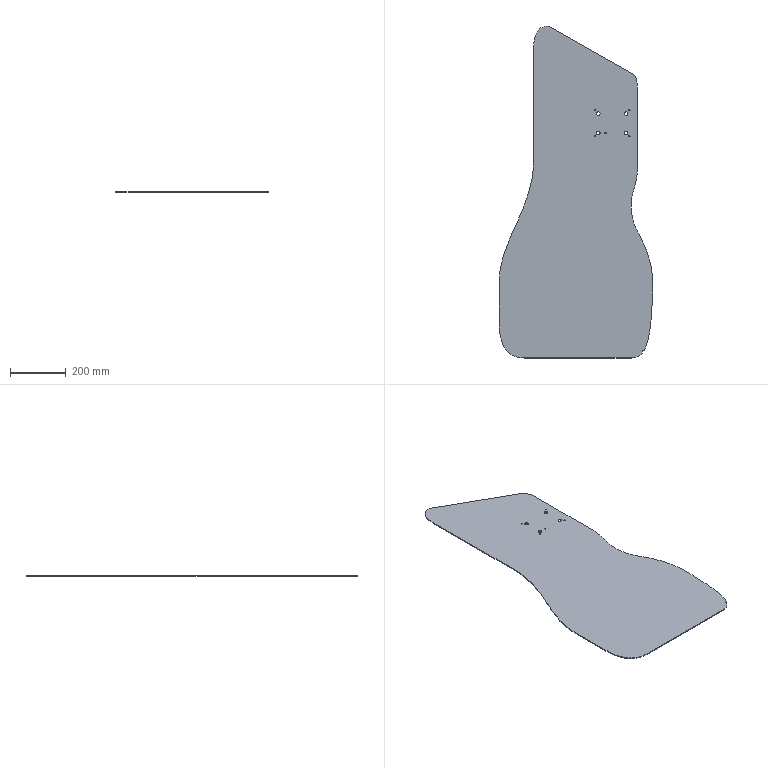Part | SolidWorks | features ICE 2, Extrusion 1 | 1 solid | 126 faces | box 552.5 x 1195 x 3 mm | volume 1469093 mm3 | plane 108 | cylinder 18 | commonest cylinder face diameters 4.5 x10 13 x8